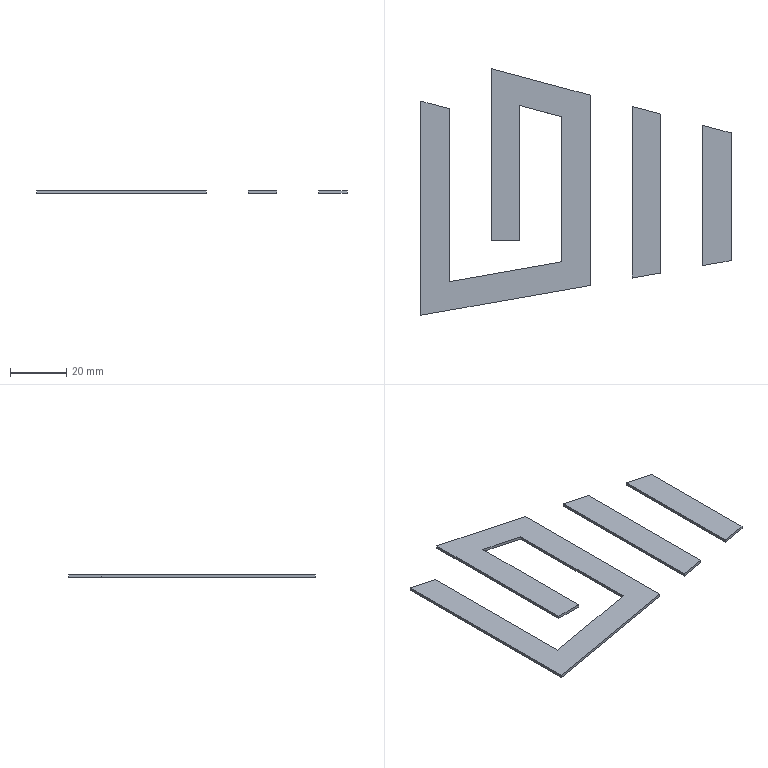Part | STEP file | COMPANY_A LOGO01001 | 3 solids | 26 faces | box 110 x 87.475 x 1 mm | volume 3655 mm3 | plane 26